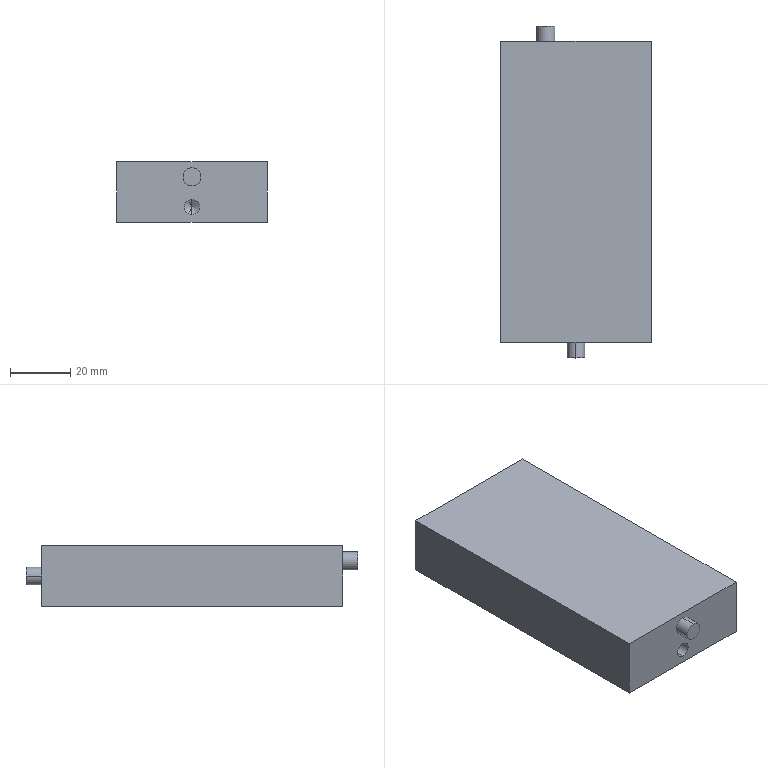Part | SolidWorks | features ICE 4, HoleWzd 3, Extrusion 1 | 1 solid | 20 faces | box 50 x 110 x 20 mm | volume 99674 mm3 | cylinder 8 | plane 8 | cone 4 | commonest cylinder face diameters 5 x4 6 x4
STEP:
#1=CARTESIAN_POINT('',(0.,85.,-2.5));
#2=VERTEX_POINT('',#1);
#3=CARTESIAN_POINT('',(0.,85.,2.5));
#4=VERTEX_POINT('',#3);
#5=CARTESIAN_POINT('',(0.,85.,0.));
#6=DIRECTION('',(0.,1.,0.));
#7=DIRECTION('',(0.,0.,1.));
#8=AXIS2_PLACEMENT_3D('',#5,#6,#7);
#9=CIRCLE('',#8,2.5);
#10=EDGE_CURVE('',#2,#4,#9,.T.);
#11=ORIENTED_EDGE('',*,*,#10,.F.);
#12=CARTESIAN_POINT('',(0.,100.,-2.5));
#13=VERTEX_POINT('',#12);
#14=CARTESIAN_POINT('',(0.,100.,-2.5));
#15=DIRECTION('',(0.,1.,0.));
#16=VECTOR('',#15,1000.);
#17=LINE('',#14,#16);
#18=EDGE_CURVE('',#2,#13,#17,.T.);
#19=ORIENTED_EDGE('',*,*,#18,.T.);
#20=CARTESIAN_POINT('',(0.,100.,2.5));
#21=VERTEX_POINT('',#20);
#22=CARTESIAN_POINT('',(0.,100.,0.));
#23=DIRECTION('',(0.,1.,0.));
#24=DIRECTION('',(0.,0.,1.));
#25=AXIS2_PLACEMENT_3D('',#22,#23,#24);
#26=CIRCLE('',#25,2.5);
#27=EDGE_CURVE('',#13,#21,#26,.T.);
#28=ORIENTED_EDGE('',*,*,#27,.T.);
#29=CARTESIAN_POINT('',(0.,100.,2.5));
#30=DIRECTION('',(0.,1.,0.));
#31=VECTOR('',#30,1000.);
#32=LINE('',#29,#31);
#33=EDGE_CURVE('',#4,#21,#32,.T.);
#34=ORIENTED_EDGE('',*,*,#33,.F.);
#35=EDGE_LOOP('',(#11,#19,#28,#34));
#36=FACE_OUTER_BOUND('',#35,.T.);
#37=CARTESIAN_POINT('',(0.,100.,0.));
#38=DIRECTION('',(0.,1.,0.));
#39=DIRECTION('',(0.,0.,1.));
#40=AXIS2_PLACEMENT_3D('',#37,#38,#39);
#41=CYLINDRICAL_SURFACE('',#40,2.5);
#42=ADVANCED_FACE('',(#36),#41,.F.);
#43=CARTESIAN_POINT('',(0.,83.498,0.));
#44=VERTEX_POINT('',#43);
#45=CARTESIAN_POINT('',(0.,85.,2.5));
#46=DIRECTION('',(0.,0.515,0.8572));
#47=VECTOR('',#46,1000.);
#48=LINE('',#45,#47);
#49=EDGE_CURVE('',#44,#4,#48,.T.);
#50=ORIENTED_EDGE('',*,*,#49,.F.);
#51=CARTESIAN_POINT('',(0.,85.,-2.5));
#52=DIRECTION('',(0.,0.515,-0.8572));
#53=VECTOR('',#52,1000.);
#54=LINE('',#51,#53);
#55=EDGE_CURVE('',#44,#2,#54,.T.);
#56=ORIENTED_EDGE('',*,*,#55,.T.);
#57=ORIENTED_EDGE('',*,*,#10,.T.);
#58=EDGE_LOOP('',(#50,#56,#57));
#59=FACE_OUTER_BOUND('',#58,.T.);
#60=CARTESIAN_POINT('',(0.,85.,0.));
#61=DIRECTION('',(0.,1.,0.));
#62=DIRECTION('',(0.,0.,1.));
#63=AXIS2_PLACEMENT_3D('',#60,#61,#62);
#64=CONICAL_SURFACE('',#63,2.5,1.03);
#65=ADVANCED_FACE('',(#59),#64,.F.);
#66=CARTESIAN_POINT('',(-13.,105.,0.));
#67=VERTEX_POINT('',#66);
#68=CARTESIAN_POINT('',(-7.,105.,0.));
#69=VERTEX_POINT('',#68);
#70=CARTESIAN_POINT('',(-10.,105.,0.));
#71=DIRECTION('',(0.,1.,0.));
#72=DIRECTION('',(-1.,0.,0.));
#73=AXIS2_PLACEMENT_3D('',#70,#71,#72);
#74=CIRCLE('',#73,3.);
#75=EDGE_CURVE('',#67,#69,#74,.T.);
#76=ORIENTED_EDGE('',*,*,#75,.F.);
#77=CARTESIAN_POINT('',(-13.,100.,0.));
#78=VERTEX_POINT('',#77);
#79=CARTESIAN_POINT('',(-13.,105.,0.));
#80=DIRECTION('',(0.,-1.,0.));
#81=VECTOR('',#80,1000.);
#82=LINE('',#79,#81);
#83=EDGE_CURVE('',#67,#78,#82,.T.);
#84=ORIENTED_EDGE('',*,*,#83,.T.);
#85=CARTESIAN_POINT('',(-7.,100.,0.));
#86=VERTEX_POINT('',#85);
#87=CARTESIAN_POINT('',(-10.,100.,0.));
#88=DIRECTION('',(0.,1.,0.));
#89=DIRECTION('',(1.,0.,0.));
#90=AXIS2_PLACEMENT_3D('',#87,#88,#89);
#91=CIRCLE('',#90,3.);
#92=EDGE_CURVE('',#78,#86,#91,.T.);
#93=ORIENTED_EDGE('',*,*,#92,.T.);
#94=CARTESIAN_POINT('',(-7.,105.,0.));
#95=DIRECTION('',(0.,-1.,0.));
#96=VECTOR('',#95,1000.);
#97=LINE('',#94,#96);
#98=EDGE_CURVE('',#69,#86,#97,.T.);
#99=ORIENTED_EDGE('',*,*,#98,.F.);
#100=EDGE_LOOP('',(#76,#84,#93,#99));
#101=FACE_OUTER_BOUND('',#100,.T.);
#102=CARTESIAN_POINT('',(-10.,105.,0.));
#103=DIRECTION('',(0.,-1.,0.));
#104=DIRECTION('',(1.,0.,0.));
#105=AXIS2_PLACEMENT_3D('',#102,#103,#104);
#106=CYLINDRICAL_SURFACE('',#105,3.);
#107=ADVANCED_FACE('',(#101),#106,.T.);
#108=CARTESIAN_POINT('',(0.,15.,-2.5));
#109=VERTEX_POINT('',#108);
#110=CARTESIAN_POINT('',(0.,15.,-7.5));
#111=VERTEX_POINT('',#110);
#112=CARTESIAN_POINT('',(0.,15.,-5.));
#113=DIRECTION('',(0.,-1.,0.));
#114=DIRECTION('',(0.,0.,-1.));
#115=AXIS2_PLACEMENT_3D('',#112,#113,#114);
#116=CIRCLE('',#115,2.5);
#117=EDGE_CURVE('',#109,#111,#116,.T.);
#118=ORIENTED_EDGE('',*,*,#117,.F.);
#119=CARTESIAN_POINT('',(0.,0.,-2.5));
#120=VERTEX_POINT('',#119);
#121=CARTESIAN_POINT('',(0.,0.,-2.5));
#122=DIRECTION('',(0.,-1.,0.));
#123=VECTOR('',#122,1000.);
#124=LINE('',#121,#123);
#125=EDGE_CURVE('',#109,#120,#124,.T.);
#126=ORIENTED_EDGE('',*,*,#125,.T.);
#127=CARTESIAN_POINT('',(0.,0.,-7.5));
#128=VERTEX_POINT('',#127);
#129=CARTESIAN_POINT('',(0.,0.,-5.));
#130=DIRECTION('',(0.,-1.,0.));
#131=DIRECTION('',(0.,0.,-1.));
#132=AXIS2_PLACEMENT_3D('',#129,#130,#131);
#133=CIRCLE('',#132,2.5);
#134=EDGE_CURVE('',#120,#128,#133,.T.);
#135=ORIENTED_EDGE('',*,*,#134,.T.);
#136=CARTESIAN_POINT('',(0.,0.,-7.5));
#137=DIRECTION('',(0.,-1.,0.));
#138=VECTOR('',#137,1000.);
#139=LINE('',#136,#138);
#140=EDGE_CURVE('',#111,#128,#139,.T.);
#141=ORIENTED_EDGE('',*,*,#140,.F.);
#142=EDGE_LOOP('',(#118,#126,#135,#141));
#143=FACE_OUTER_BOUND('',#142,.T.);
#144=CARTESIAN_POINT('',(0.,0.,-5.));
#145=DIRECTION('',(0.,-1.,0.));
#146=DIRECTION('',(0.,0.,-1.));
#147=AXIS2_PLACEMENT_3D('',#144,#145,#146);
#148=CYLINDRICAL_SURFACE('',#147,2.5);
#149=ADVANCED_FACE('',(#143),#148,.F.);
#150=CARTESIAN_POINT('',(0.,16.502,-5.));
#151=VERTEX_POINT('',#150);
#152=CARTESIAN_POINT('',(0.,15.,-7.5));
#153=DIRECTION('',(0.,-0.515,-0.8572));
#154=VECTOR('',#153,1000.);
#155=LINE('',#152,#154);
#156=EDGE_CURVE('',#151,#111,#155,.T.);
#157=ORIENTED_EDGE('',*,*,#156,.F.);
#158=CARTESIAN_POINT('',(0.,15.,-2.5));
#159=DIRECTION('',(0.,-0.515,0.8572));
#160=VECTOR('',#159,1000.);
#161=LINE('',#158,#160);
#162=EDGE_CURVE('',#151,#109,#161,.T.);
#163=ORIENTED_EDGE('',*,*,#162,.T.);
#164=ORIENTED_EDGE('',*,*,#117,.T.);
#165=EDGE_LOOP('',(#157,#163,#164));
#166=FACE_OUTER_BOUND('',#165,.T.);
#167=CARTESIAN_POINT('',(0.,15.,-5.));
#168=DIRECTION('',(0.,-1.,0.));
#169=DIRECTION('',(0.,0.,-1.));
#170=AXIS2_PLACEMENT_3D('',#167,#168,#169);
#171=CONICAL_SURFACE('',#170,2.5,1.03);
#172=ADVANCED_FACE('',(#166),#171,.F.);
#173=CARTESIAN_POINT('',(0.,-5.,2.));
#174=VERTEX_POINT('',#173);
#175=CARTESIAN_POINT('',(0.,-5.,8.));
#176=VERTEX_POINT('',#175);
#177=CARTESIAN_POINT('',(0.,-5.,5.));
#178=DIRECTION('',(0.,-1.,0.));
#179=DIRECTION('',(0.,0.,-1.));
#180=AXIS2_PLACEMENT_3D('',#177,#178,#179);
#181=CIRCLE('',#180,3.);
#182=EDGE_CURVE('',#174,#176,#181,.T.);
#183=ORIENTED_EDGE('',*,*,#182,.F.);
#184=CARTESIAN_POINT('',(0.,0.,2.));
#185=VERTEX_POINT('',#184);
#186=CARTESIAN_POINT('',(0.,-5.,2.));
#187=DIRECTION('',(0.,1.,0.));
#188=VECTOR('',#187,1000.);
#189=LINE('',#186,#188);
#190=EDGE_CURVE('',#174,#185,#189,.T.);
#191=ORIENTED_EDGE('',*,*,#190,.T.);
#192=CARTESIAN_POINT('',(0.,0.,8.));
#193=VERTEX_POINT('',#192);
#194=CARTESIAN_POINT('',(0.,0.,5.));
#195=DIRECTION('',(0.,-1.,0.));
#196=DIRECTION('',(0.,0.,-1.));
#197=AXIS2_PLACEMENT_3D('',#194,#195,#196);
#198=CIRCLE('',#197,3.);
#199=EDGE_CURVE('',#185,#193,#198,.T.);
#200=ORIENTED_EDGE('',*,*,#199,.T.);
#201=CARTESIAN_POINT('',(0.,-5.,8.));
#202=DIRECTION('',(0.,1.,0.));
#203=VECTOR('',#202,1000.);
#204=LINE('',#201,#203);
#205=EDGE_CURVE('',#176,#193,#204,.T.);
#206=ORIENTED_EDGE('',*,*,#205,.F.);
#207=EDGE_LOOP('',(#183,#191,#200,#206));
#208=FACE_OUTER_BOUND('',#207,.T.);
#209=CARTESIAN_POINT('',(0.,-5.,5.));
#210=DIRECTION('',(0.,1.,0.));
#211=DIRECTION('',(0.,0.,1.));
#212=AXIS2_PLACEMENT_3D('',#209,#210,#211);
#213=CYLINDRICAL_SURFACE('',#212,3.);
#214=ADVANCED_FACE('',(#208),#213,.T.);
#215=CARTESIAN_POINT('',(25.,100.,-10.));
#216=VERTEX_POINT('',#215);
#217=CARTESIAN_POINT('',(25.,0.,-10.));
#218=VERTEX_POINT('',#217);
#219=CARTESIAN_POINT('',(25.,100.,-10.));
#220=DIRECTION('',(0.,-1.,0.));
#221=VECTOR('',#220,1000.);
#222=LINE('',#219,#221);
#223=EDGE_CURVE('',#216,#218,#222,.T.);
#224=ORIENTED_EDGE('',*,*,#223,.F.);
#225=CARTESIAN_POINT('',(25.,100.,10.));
#226=VERTEX_POINT('',#225);
#227=CARTESIAN_POINT('',(25.,100.,-10.));
#228=DIRECTION('',(0.,0.,1.));
#229=VECTOR('',#228,1000.);
#230=LINE('',#227,#229);
#231=EDGE_CURVE('',#216,#226,#230,.T.);
#232=ORIENTED_EDGE('',*,*,#231,.T.);
#233=CARTESIAN_POINT('',(25.,0.,10.));
#234=VERTEX_POINT('',#233);
#235=CARTESIAN_POINT('',(25.,100.,10.));
#236=DIRECTION('',(0.,-1.,0.));
#237=VECTOR('',#236,1000.);
#238=LINE('',#235,#237);
#239=EDGE_CURVE('',#226,#234,#238,.T.);
#240=ORIENTED_EDGE('',*,*,#239,.T.);
#241=CARTESIAN_POINT('',(25.,0.,10.));
#242=DIRECTION('',(0.,0.,-1.));
#243=VECTOR('',#242,1000.);
#244=LINE('',#241,#243);
#245=EDGE_CURVE('',#234,#218,#244,.T.);
#246=ORIENTED_EDGE('',*,*,#245,.T.);
#247=EDGE_LOOP('',(#224,#232,#240,#246));
#248=FACE_OUTER_BOUND('',#247,.T.);
#249=CARTESIAN_POINT('',(25.,100.,10.));
#250=DIRECTION('',(-1.,0.,0.));
#251=DIRECTION('',(0.,0.,1.));
#252=AXIS2_PLACEMENT_3D('',#249,#250,#251);
#253=PLANE('',#252);
#254=ADVANCED_FACE('',(#248),#253,.F.);
#255=CARTESIAN_POINT('',(-25.,100.,-10.));
#256=VERTEX_POINT('',#255);
#257=CARTESIAN_POINT('',(-25.,0.,-10.));
#258=VERTEX_POINT('',#257);
#259=CARTESIAN_POINT('',(-25.,100.,-10.));
#260=DIRECTION('',(0.,-1.,0.));
#261=VECTOR('',#260,1000.);
#262=LINE('',#259,#261);
#263=EDGE_CURVE('',#256,#258,#262,.T.);
#264=ORIENTED_EDGE('',*,*,#263,.F.);
#265=CARTESIAN_POINT('',(25.,100.,-10.));
#266=DIRECTION('',(1.,0.,0.));
#267=VECTOR('',#266,1000.);
#268=LINE('',#265,#267);
#269=EDGE_CURVE('',#256,#216,#268,.T.);
#270=ORIENTED_EDGE('',*,*,#269,.T.);
#271=ORIENTED_EDGE('',*,*,#223,.T.);
#272=CARTESIAN_POINT('',(-25.,0.,-10.));
#273=DIRECTION('',(-1.,0.,0.));
#274=VECTOR('',#273,1000.);
#275=LINE('',#272,#274);
#276=EDGE_CURVE('',#218,#258,#275,.T.);
#277=ORIENTED_EDGE('',*,*,#276,.T.);
#278=EDGE_LOOP('',(#264,#270,#271,#277));
#279=FACE_OUTER_BOUND('',#278,.T.);
#280=CARTESIAN_POINT('',(-25.,100.,-10.));
#281=DIRECTION('',(0.,0.,1.));
#282=DIRECTION('',(1.,0.,0.));
#283=AXIS2_PLACEMENT_3D('',#280,#281,#282);
#284=PLANE('',#283);
#285=ADVANCED_FACE('',(#279),#284,.F.);
#286=CARTESIAN_POINT('',(-25.,0.,10.));
#287=VERTEX_POINT('',#286);
#288=CARTESIAN_POINT('',(-25.,0.,10.));
#289=DIRECTION('',(0.,0.,1.));
#290=VECTOR('',#289,1000.);
#291=LINE('',#288,#290);
#292=EDGE_CURVE('',#258,#287,#291,.T.);
#293=ORIENTED_EDGE('',*,*,#292,.T.);
#294=CARTESIAN_POINT('',(-25.,100.,10.));
#295=VERTEX_POINT('',#294);
#296=CARTESIAN_POINT('',(-25.,100.,10.));
#297=DIRECTION('',(0.,-1.,0.));
#298=VECTOR('',#297,1000.);
#299=LINE('',#296,#298);
#300=EDGE_CURVE('',#295,#287,#299,.T.);
#301=ORIENTED_EDGE('',*,*,#300,.F.);
#302=CARTESIAN_POINT('',(-25.,100.,10.));
#303=DIRECTION('',(0.,0.,1.));
#304=VECTOR('',#303,1000.);
#305=LINE('',#302,#304);
#306=EDGE_CURVE('',#256,#295,#305,.T.);
#307=ORIENTED_EDGE('',*,*,#306,.F.);
#308=ORIENTED_EDGE('',*,*,#263,.T.);
#309=EDGE_LOOP('',(#293,#301,#307,#308));
#310=FACE_OUTER_BOUND('',#309,.T.);
#311=CARTESIAN_POINT('',(-25.,100.,10.));
#312=DIRECTION('',(1.,0.,0.));
#313=DIRECTION('',(0.,0.,-1.));
#314=AXIS2_PLACEMENT_3D('',#311,#312,#313);
#315=PLANE('',#314);
#316=ADVANCED_FACE('',(#310),#315,.F.);
#317=ORIENTED_EDGE('',*,*,#239,.F.);
#318=CARTESIAN_POINT('',(25.,100.,10.));
#319=DIRECTION('',(1.,0.,0.));
#320=VECTOR('',#319,1000.);
#321=LINE('',#318,#320);
#322=EDGE_CURVE('',#295,#226,#321,.T.);
#323=ORIENTED_EDGE('',*,*,#322,.F.);
#324=ORIENTED_EDGE('',*,*,#300,.T.);
#325=CARTESIAN_POINT('',(-25.,0.,10.));
#326=DIRECTION('',(1.,0.,0.));
#327=VECTOR('',#326,1000.);
#328=LINE('',#325,#327);
#329=EDGE_CURVE('',#287,#234,#328,.T.);
#330=ORIENTED_EDGE('',*,*,#329,.T.);
#331=EDGE_LOOP('',(#317,#323,#324,#330));
#332=FACE_OUTER_BOUND('',#331,.T.);
#333=CARTESIAN_POINT('',(-25.,100.,10.));
#334=DIRECTION('',(0.,0.,-1.));
#335=DIRECTION('',(-1.,0.,0.));
#336=AXIS2_PLACEMENT_3D('',#333,#334,#335);
#337=PLANE('',#336);
#338=ADVANCED_FACE('',(#332),#337,.F.);
#339=CARTESIAN_POINT('',(0.,0.,-5.));
#340=DIRECTION('',(0.,-1.,0.));
#341=DIRECTION('',(0.,0.,-1.));
#342=AXIS2_PLACEMENT_3D('',#339,#340,#341);
#343=CIRCLE('',#342,2.5);
#344=EDGE_CURVE('',#128,#120,#343,.T.);
#345=ORIENTED_EDGE('',*,*,#344,.F.);
#346=ORIENTED_EDGE('',*,*,#134,.F.);
#347=EDGE_LOOP('',(#345,#346));
#348=FACE_BOUND('',#347,.T.);
#349=CARTESIAN_POINT('',(0.,0.,5.));
#350=DIRECTION('',(0.,-1.,0.));
#351=DIRECTION('',(0.,0.,-1.));
#352=AXIS2_PLACEMENT_3D('',#349,#350,#351);
#353=CIRCLE('',#352,3.);
#354=EDGE_CURVE('',#193,#185,#353,.T.);
#355=ORIENTED_EDGE('',*,*,#354,.F.);
#356=ORIENTED_EDGE('',*,*,#199,.F.);
#357=EDGE_LOOP('',(#355,#356));
#358=FACE_BOUND('',#357,.T.);
#359=ORIENTED_EDGE('',*,*,#245,.F.);
#360=ORIENTED_EDGE('',*,*,#329,.F.);
#361=ORIENTED_EDGE('',*,*,#292,.F.);
#362=ORIENTED_EDGE('',*,*,#276,.F.);
#363=EDGE_LOOP('',(#359,#360,#361,#362));
#364=FACE_OUTER_BOUND('',#363,.T.);
#365=CARTESIAN_POINT('',(0.,0.,0.));
#366=DIRECTION('',(0.,-1.,0.));
#367=DIRECTION('',(0.,0.,-1.));
#368=AXIS2_PLACEMENT_3D('',#365,#366,#367);
#369=PLANE('',#368);
#370=ADVANCED_FACE('',(#348,#358,#364),#369,.T.);
#371=ORIENTED_EDGE('',*,*,#190,.F.);
#372=CARTESIAN_POINT('',(0.,-5.,5.));
#373=DIRECTION('',(0.,-1.,0.));
#374=DIRECTION('',(0.,0.,-1.));
#375=AXIS2_PLACEMENT_3D('',#372,#373,#374);
#376=CIRCLE('',#375,3.);
#377=EDGE_CURVE('',#176,#174,#376,.T.);
#378=ORIENTED_EDGE('',*,*,#377,.F.);
#379=ORIENTED_EDGE('',*,*,#205,.T.);
#380=ORIENTED_EDGE('',*,*,#354,.T.);
#381=EDGE_LOOP('',(#371,#378,#379,#380));
#382=FACE_OUTER_BOUND('',#381,.T.);
#383=CARTESIAN_POINT('',(0.,-5.,5.));
#384=DIRECTION('',(0.,1.,0.));
#385=DIRECTION('',(0.,0.,1.));
#386=AXIS2_PLACEMENT_3D('',#383,#384,#385);
#387=CYLINDRICAL_SURFACE('',#386,3.);
#388=ADVANCED_FACE('',(#382),#387,.T.);
#389=ORIENTED_EDGE('',*,*,#377,.T.);
#390=ORIENTED_EDGE('',*,*,#182,.T.);
#391=EDGE_LOOP('',(#389,#390));
#392=FACE_OUTER_BOUND('',#391,.T.);
#393=CARTESIAN_POINT('',(0.,-5.,5.));
#394=DIRECTION('',(0.,-1.,0.));
#395=DIRECTION('',(0.,0.,-1.));
#396=AXIS2_PLACEMENT_3D('',#393,#394,#395);
#397=PLANE('',#396);
#398=ADVANCED_FACE('',(#392),#397,.T.);
#399=ORIENTED_EDGE('',*,*,#162,.F.);
#400=ORIENTED_EDGE('',*,*,#156,.T.);
#401=CARTESIAN_POINT('',(0.,15.,-5.));
#402=DIRECTION('',(0.,-1.,0.));
#403=DIRECTION('',(0.,0.,-1.));
#404=AXIS2_PLACEMENT_3D('',#401,#402,#403);
#405=CIRCLE('',#404,2.5);
#406=EDGE_CURVE('',#111,#109,#405,.T.);
#407=ORIENTED_EDGE('',*,*,#406,.T.);
#408=EDGE_LOOP('',(#399,#400,#407));
#409=FACE_OUTER_BOUND('',#408,.T.);
#410=CARTESIAN_POINT('',(0.,15.,-5.));
#411=DIRECTION('',(0.,-1.,0.));
#412=DIRECTION('',(0.,0.,-1.));
#413=AXIS2_PLACEMENT_3D('',#410,#411,#412);
#414=CONICAL_SURFACE('',#413,2.5,1.03);
#415=ADVANCED_FACE('',(#409),#414,.F.);
#416=ORIENTED_EDGE('',*,*,#125,.F.);
#417=ORIENTED_EDGE('',*,*,#406,.F.);
#418=ORIENTED_EDGE('',*,*,#140,.T.);
#419=ORIENTED_EDGE('',*,*,#344,.T.);
#420=EDGE_LOOP('',(#416,#417,#418,#419));
#421=FACE_OUTER_BOUND('',#420,.T.);
#422=CARTESIAN_POINT('',(0.,0.,-5.));
#423=DIRECTION('',(0.,-1.,0.));
#424=DIRECTION('',(0.,0.,-1.));
#425=AXIS2_PLACEMENT_3D('',#422,#423,#424);
#426=CYLINDRICAL_SURFACE('',#425,2.5);
#427=ADVANCED_FACE('',(#421),#426,.F.);
#428=CARTESIAN_POINT('',(0.,100.,0.));
#429=DIRECTION('',(0.,1.,0.));
#430=DIRECTION('',(0.,0.,1.));
#431=AXIS2_PLACEMENT_3D('',#428,#429,#430);
#432=CIRCLE('',#431,2.5);
#433=EDGE_CURVE('',#21,#13,#432,.T.);
#434=ORIENTED_EDGE('',*,*,#433,.F.);
#435=ORIENTED_EDGE('',*,*,#27,.F.);
#436=EDGE_LOOP('',(#434,#435));
#437=FACE_BOUND('',#436,.T.);
#438=CARTESIAN_POINT('',(-10.,100.,0.));
#439=DIRECTION('',(0.,1.,0.));
#440=DIRECTION('',(1.,0.,0.));
#441=AXIS2_PLACEMENT_3D('',#438,#439,#440);
#442=CIRCLE('',#441,3.);
#443=EDGE_CURVE('',#86,#78,#442,.T.);
#444=ORIENTED_EDGE('',*,*,#443,.F.);
#445=ORIENTED_EDGE('',*,*,#92,.F.);
#446=EDGE_LOOP('',(#444,#445));
#447=FACE_BOUND('',#446,.T.);
#448=ORIENTED_EDGE('',*,*,#322,.T.);
#449=ORIENTED_EDGE('',*,*,#231,.F.);
#450=ORIENTED_EDGE('',*,*,#269,.F.);
#451=ORIENTED_EDGE('',*,*,#306,.T.);
#452=EDGE_LOOP('',(#448,#449,#450,#451));
#453=FACE_OUTER_BOUND('',#452,.T.);
#454=CARTESIAN_POINT('',(25.,100.,-10.));
#455=DIRECTION('',(0.,-1.,0.));
#456=DIRECTION('',(1.,0.,0.));
#457=AXIS2_PLACEMENT_3D('',#454,#455,#456);
#458=PLANE('',#457);
#459=ADVANCED_FACE('',(#437,#447,#453),#458,.F.);
#460=ORIENTED_EDGE('',*,*,#83,.F.);
#461=CARTESIAN_POINT('',(-10.,105.,0.));
#462=DIRECTION('',(0.,1.,0.));
#463=DIRECTION('',(-1.,0.,0.));
#464=AXIS2_PLACEMENT_3D('',#461,#462,#463);
#465=CIRCLE('',#464,3.);
#466=EDGE_CURVE('',#69,#67,#465,.T.);
#467=ORIENTED_EDGE('',*,*,#466,.F.);
#468=ORIENTED_EDGE('',*,*,#98,.T.);
#469=ORIENTED_EDGE('',*,*,#443,.T.);
#470=EDGE_LOOP('',(#460,#467,#468,#469));
#471=FACE_OUTER_BOUND('',#470,.T.);
#472=CARTESIAN_POINT('',(-10.,105.,0.));
#473=DIRECTION('',(0.,-1.,0.));
#474=DIRECTION('',(1.,0.,0.));
#475=AXIS2_PLACEMENT_3D('',#472,#473,#474);
#476=CYLINDRICAL_SURFACE('',#475,3.);
#477=ADVANCED_FACE('',(#471),#476,.T.);
#478=ORIENTED_EDGE('',*,*,#466,.T.);
#479=ORIENTED_EDGE('',*,*,#75,.T.);
#480=EDGE_LOOP('',(#478,#479));
#481=FACE_OUTER_BOUND('',#480,.T.);
#482=CARTESIAN_POINT('',(-10.,105.,0.));
#483=DIRECTION('',(0.,1.,0.));
#484=DIRECTION('',(-1.,0.,0.));
#485=AXIS2_PLACEMENT_3D('',#482,#483,#484);
#486=PLANE('',#485);
#487=ADVANCED_FACE('',(#481),#486,.T.);
#488=ORIENTED_EDGE('',*,*,#55,.F.);
#489=ORIENTED_EDGE('',*,*,#49,.T.);
#490=CARTESIAN_POINT('',(0.,85.,0.));
#491=DIRECTION('',(0.,1.,0.));
#492=DIRECTION('',(0.,0.,1.));
#493=AXIS2_PLACEMENT_3D('',#490,#491,#492);
#494=CIRCLE('',#493,2.5);
#495=EDGE_CURVE('',#4,#2,#494,.T.);
#496=ORIENTED_EDGE('',*,*,#495,.T.);
#497=EDGE_LOOP('',(#488,#489,#496));
#498=FACE_OUTER_BOUND('',#497,.T.);
#499=CARTESIAN_POINT('',(0.,85.,0.));
#500=DIRECTION('',(0.,1.,0.));
#501=DIRECTION('',(0.,0.,1.));
#502=AXIS2_PLACEMENT_3D('',#499,#500,#501);
#503=CONICAL_SURFACE('',#502,2.5,1.03);
#504=ADVANCED_FACE('',(#498),#503,.F.);
#505=ORIENTED_EDGE('',*,*,#18,.F.);
#506=ORIENTED_EDGE('',*,*,#495,.F.);
#507=ORIENTED_EDGE('',*,*,#33,.T.);
#508=ORIENTED_EDGE('',*,*,#433,.T.);
#509=EDGE_LOOP('',(#505,#506,#507,#508));
#510=FACE_OUTER_BOUND('',#509,.T.);
#511=CARTESIAN_POINT('',(0.,100.,0.));
#512=DIRECTION('',(0.,1.,0.));
#513=DIRECTION('',(0.,0.,1.));
#514=AXIS2_PLACEMENT_3D('',#511,#512,#513);
#515=CYLINDRICAL_SURFACE('',#514,2.5);
#516=ADVANCED_FACE('',(#510),#515,.F.);
#517=CLOSED_SHELL('',(#42,#65,#107,#149,#172,#214,#254,#285,#316,#338,#370,#388,#398,#415,#427,#459,#477,#487,#504,#516));
#518=MANIFOLD_SOLID_BREP('',#517);
#519=CARTESIAN_POINT('',(0.,0.,0.));
#520=DIRECTION('',(0.,0.,1.));
#521=DIRECTION('',(1.,0.,0.));
#522=AXIS2_PLACEMENT_3D('',#519,#520,#521);
#523=(LENGTH_UNIT()NAMED_UNIT(*)SI_UNIT(.MILLI.,.METRE.));
#524=UNCERTAINTY_MEASURE_WITH_UNIT(LENGTH_MEASURE(0.00001),#523,'','');
#525=(NAMED_UNIT(*)PLANE_ANGLE_UNIT()SI_UNIT($,.RADIAN.));
#526=(NAMED_UNIT(*)SI_UNIT($,.STERADIAN.)SOLID_ANGLE_UNIT());
#527=(GEOMETRIC_REPRESENTATION_CONTEXT(3)GLOBAL_UNCERTAINTY_ASSIGNED_CONTEXT((#524))GLOBAL_UNIT_ASSIGNED_CONTEXT((#523,#525,#526))REPRESENTATION_CONTEXT('',''));
#528=ADVANCED_BREP_SHAPE_REPRESENTATION('',(#518,#522),#527);